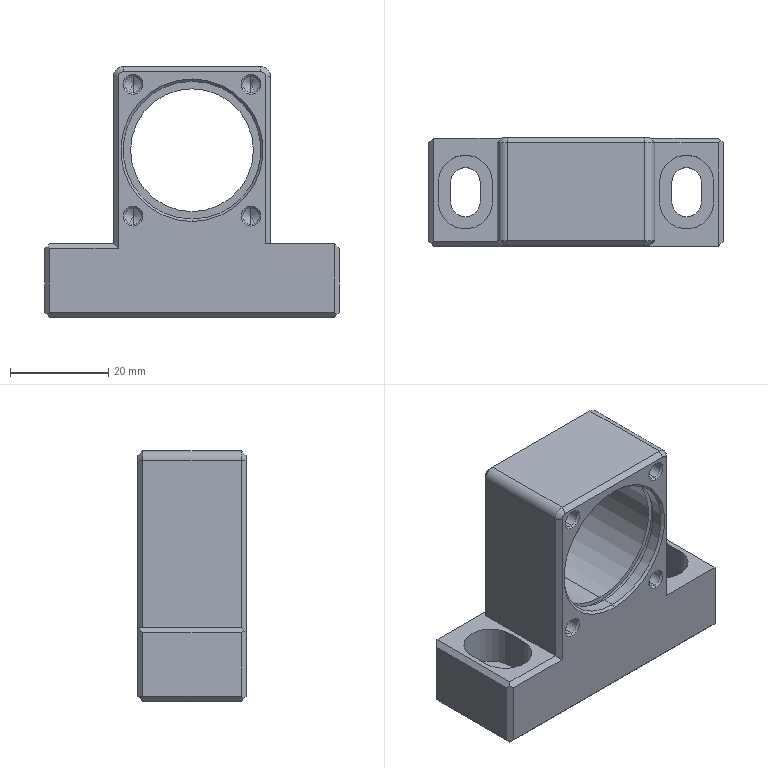Part | NX | features BREP 1 | 1 solid | 90 faces | box 60 x 22 x 51 mm | volume 28131 mm3 | plane 42 | cylinder 26 | cone 22 | commonest cylinder face diameters 3.3 x8 6 x4 11 x4 28 x4 4 x2 25 x2